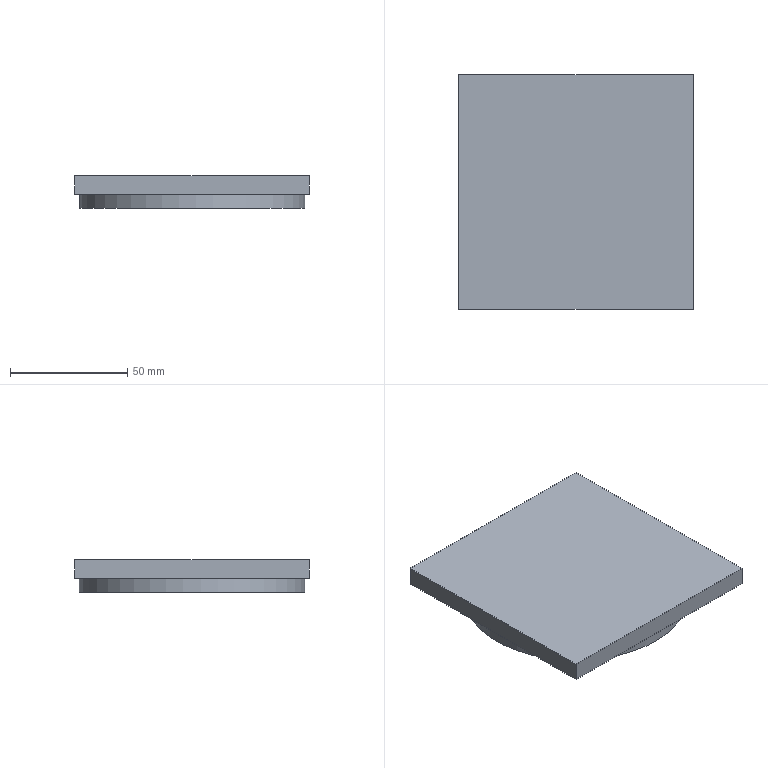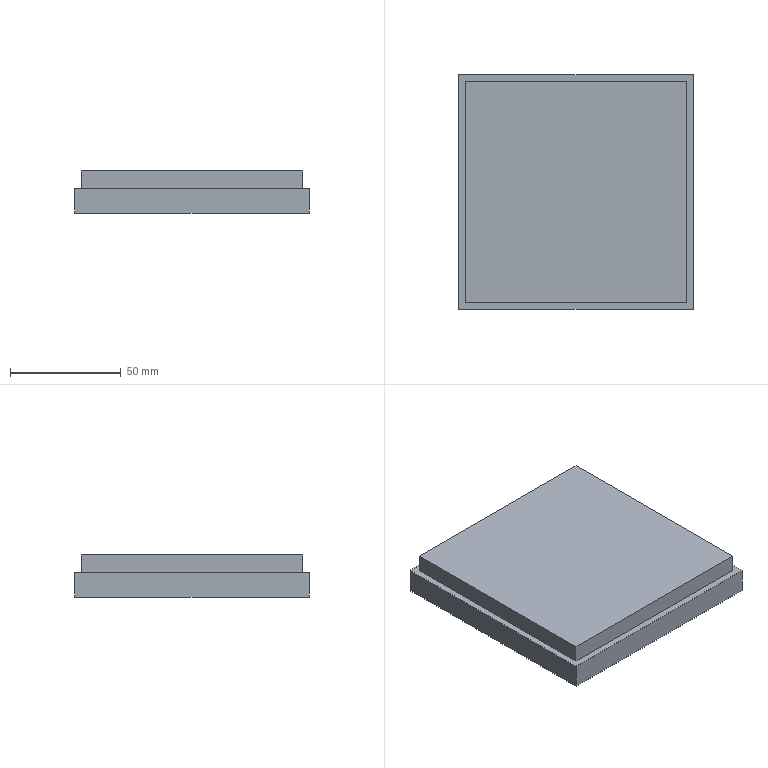CAM job | NX | 3-axis milling, drilling | part box 100 x 100 x 14 mm | stock box 106 x 106 x 19 mm
Tools:
number,name,description,diameter,corner_radius,flute_length,length,flutes
1,FACEMILL-60,Milling Tool-5 Parameters,60.0,0.0,50.0,75.0,2
2,D-12,Milling Tool-5 Parameters,12.0,0.0,50.0,75.0,2
3,D-6,Milling Tool-5 Parameters,6.0,0.0,50.0,75.0,2
4,SPOTDRILL-D8,Spot Drill,8.0,4.0,0.0,100.0,2
5,DRILL-4.3,Spot Drill,4.3,2.15,0.0,100.0,2
6,DRILL-5.5,Spot Drill,5.5,2.75,0.0,100.0,2
7,D10,Milling Tool-5 Parameters,10.0,0.0,50.0,75.0,2
Operations:
program,operation,operation_type,tool,method,geometry_group,spindle_rpm,surface_speed,feed_per_tooth,feed_cut,feed_plunge,cut_length_mm,path_length_mm,cut_time_min,machine_time_min
PROGRAM,FLOOR_FACING,VolumeBased25DMillingOperation,FACEMILL-60,METHOD,WORKPIECE,4000.0,753.0,0.1,800.0,100.0,356.0,724.579,0.445,0.4819
PROGRAM,ADAPTIVE_MILLING,CavityMilling,D-12,METHOD,WORKPIECE,6000.0,226.0,0.3333,4000.0,100.0,8890.693,9162.868,1.758,1.785
PROGRAM,PLANAR_MILL,PlanarMilling,D-6,METHOD,WORKPIECE,4500.0,84.0,0.1111,1000.0,100.0,401.438,838.455,0.4014,0.4451
PROGRAM,SPOT_DRILLING,HoleDrilling,SPOTDRILL-D8,METHOD,WORKPIECE,2000.0,50.0,0.05,200.0,100.0,34.5,478.953,0.1725,0.2169
PROGRAM,SPOT_DRILLING_COPY,HoleDrilling,SPOTDRILL-D8,METHOD,WORKPIECE,2000.0,50.0,0.05,200.0,100.0,61.8,765.8,0.309,0.3794
PROGRAM,DRILLING,HoleDrilling,DRILL-4.3,METHOD,WORKPIECE,2000.0,27.0,0.05,200.0,0.0,526.292,1230.292,0.3786,0.449
PROGRAM,DRILLING_COPY,HoleDrilling,DRILL-5.5,METHOD,WORKPIECE,2000.0,27.0,0.05,200.0,0.0,123.0,567.453,0.1313,0.1757
PROGRAM,PLANAR_MILL_2,PlanarMilling,SPOTDRILL-D8,METHOD,WORKPIECE,3000.0,75.0,0.25,1500.0,100.0,330.368,428.368,0.2202,0.23
PROGRAM,PLANAR_MILL_2_COPY,PlanarMilling,SPOTDRILL-D8,METHOD,WORKPIECE,3000.0,75.0,0.0833,500.0,100.0,102.823,533.396,0.2056,0.2487
PROGRAM,PLANAR_MILL_2_COPY_COPY,PlanarMilling,SPOTDRILL-D8,METHOD,WORKPIECE,3000.0,75.0,0.0833,500.0,100.0,151.456,248.456,0.3029,0.3126
PROGRAM,PLANAR_MILL_COPY,PlanarMilling,D-6,METHOD,WORKPIECE,4500.0,84.0,0.0222,200.0,100.0,74.549,516.482,0.3727,0.4169
PROGRAM,PLANAR_MILL_1,PlanarMilling,D10,METHOD,WORKPIECE,4500.0,141.0,0.1111,1000.0,100.0,353.223,461.223,0.3532,0.364
PROGRAM,PLANAR_MILL_1_COPY,PlanarMilling,D10,METHOD,WORKPIECE,4500.0,141.0,0.1111,1000.0,100.0,140.89,248.89,0.1409,0.1517
PROGRAM_1,ADAPTIVE_MILLING_1_COPY,CavityMilling,D-12,METHOD,WORKPIECE_2,6000.0,226.0,0.3333,4000.0,100.0,2371.58,2386.48,0.5929,0.5944
PROGRAM_1,ADAPTIVE_MILLING_1,CavityMilling,D-12,METHOD,WORKPIECE_2,6000.0,226.0,0.3333,4000.0,100.0,6972.461,6996.261,1.743,1.746
PROGRAM_1,FLOOR_FACING_1,VolumeBased25DMillingOperation,FACEMILL-60,METHOD,MCS-2,4000.0,1005.0,0.0625,500.0,100.0,370.672,599.567,0.7413,0.7642
PROGRAM_1,PLANAR_MILL_2_COPY_1,PlanarMilling,SPOTDRILL-D8,METHOD,WORKPIECE_2,3000.0,75.0,0.25,1500.0,100.0,158.812,175.812,0.1059,0.1076
PROGRAM_1,PLANAR_MILL_2_COPY_1_COPY,PlanarMilling,SPOTDRILL-D8,METHOD,WORKPIECE_2,3000.0,75.0,0.25,1500.0,100.0,327.226,344.226,0.2182,0.2199
FIXTURE,ADAPTIVE_MILLING_2,CavityMilling,D-12,METHOD,WORKPIECE_-3,4500.0,169.0,0.2222,2000.0,100.0,7576.188,7594.288,3.788,3.79
FIXTURE,FLOOR_FACING_2,VolumeBased25DMillingOperation,D-12,METHOD,WORKPIECE_-3,4500.0,100.0,0.1178,1000.0,100.0,790.841,816.041,0.7908,0.7934
FIXTURE,PLANAR_MILL_4,PlanarMilling,D-12,METHOD,WORKPIECE_-3,4500.0,100.0,0.1178,500.0,100.0,282.051,301.091,0.5641,0.566